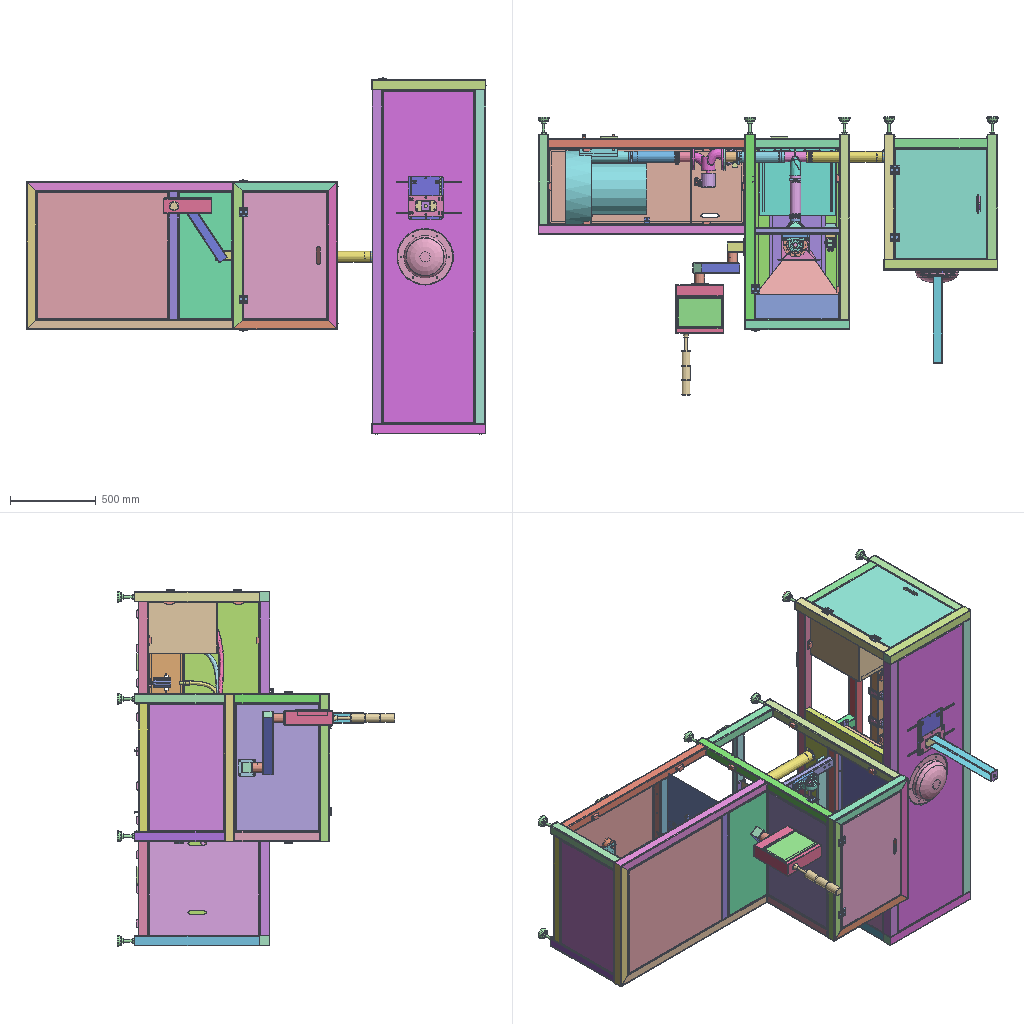Assembly | STEP file | 143 different items | 370 placed | box 2675 x 1617 x 2074 mm
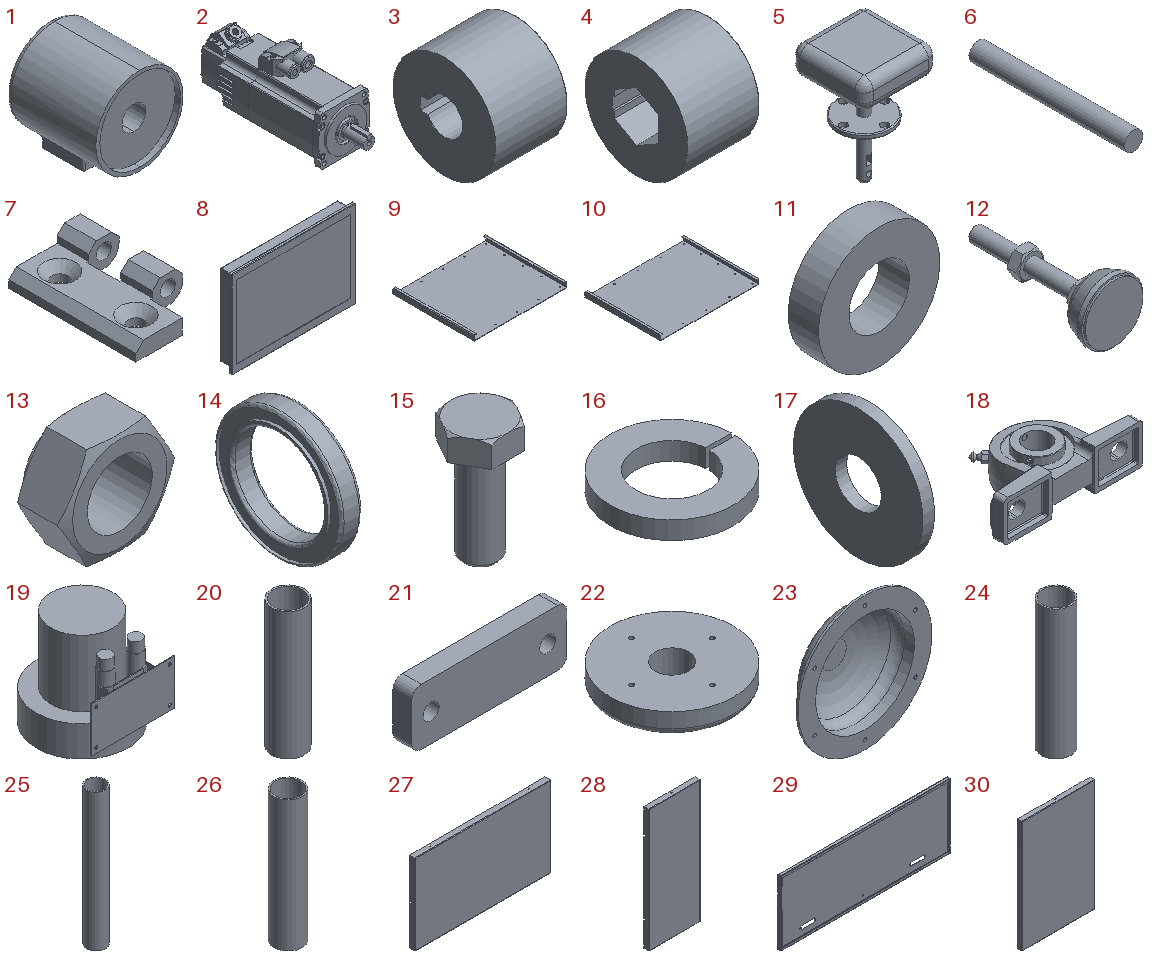Parts list (item | name | quantity | parent item | size | volume):
1 | - | x1 | - | 80 x 82 x 92.2 mm | 393243 mm3
2 | 400W (brake)_1FL60342AF211AB1 | x2 | in JBJ-P-1019-00 | 63.062 x 188.688 x 80 mm | 431591 mm3
3 | ATP40XL050-B-N14 | x1 | in JBJ-P-1019-00 | 28 x 40 x 40 mm | 30210 mm3
4 | ATP40XL050-B-hex socket | x1 | in JBJ-P-1002-00 | 28 x 40 x 40 mm | 27766 mm3
5 | Anemometer | x1 | in Test rig | 80 x 80 x 130 mm | 198324 mm3
6 | C_HHSZ50_pin | x7 | in Hinge 50-hole 30X30_C-HHSZ50 | 6 x 50 x 6 mm | 1414 mm3
7 | C_HHSZ50_pr | x14 | in Hinge 50-hole 30X30_C-HHSZ50 | 31 x 50 x 11.5 mm | 6935 mm3
8 | Display screen | x1 | in Test rig | 274 x 42.7 x 193 mm | 1730721 mm3
9 | Electrical box base plate | x1 | in Test rig | 408 x 355 x 23 mm | 248875 mm3
10 | Electrical box base plate 2 | x1 | in Test rig | 453 x 345 x 23 mm | 265143 mm3
11 | Fixed ring | x1 | in Test rig | 40 x 10 x 40 mm | 9425 mm3
12 | Foot cup | x10 | in JBJ-P-1006-00, Test rig | 65 x 147 x 65 mm | 56921 mm3
13 | GB13681-1992 nut M6 | x8 | in Test rig | 10.835 x 5 x 9.372 mm | 219.571 mm3
14 | GB276-1994 bearing 61806-2Z | x2 | in JBJ-P-1002-00 | 7 x 42 x 42 mm | 3844 mm3
15 | GB5783-2000 bolt M6X16 | x2 | in JBJ-P-1019-00 | 10.89 x 9.431 x 20 mm | 757.875 mm3
16 | GB93-1987 washer 6 | x2 | in JBJ-P-1019-00 | 10.997 x 11 x 1.6 mm | 99.231 mm3
17 | GB96.1-2002 washer 6 | x1 | in JBJ-P-1019-00 | 1.6 x 18 x 18 mm | 355.679 mm3
18 | GBT7810-1995-UCP206 | x3 | in JBJ-P-1002-00 | 165 x 84.83 x 48 mm | 210278 mm3
19 | High-pressure fan RB-81D-2  5.5 | x1 | in Test rig | 445 x 470 x 470 mm | 48196616 mm3
20 | JBJ-P-1000-01 | x1 | in JBJ-P-1000-00 | 64 x 64 x 250 mm | 143728 mm3
21 | JBJ-P-1000-03 | x3 | in JBJ-P-1000-00, Test rig | 165 x 20 x 60 mm | 187204 mm3
22 | JBJ-P-1000-04 | x1 | in Test rig | 198 x 198 x 55 mm | 1265765 mm3
23 | JBJ-P-1000-05 | x1 | in Test rig | 322 x 80 x 322 mm | 568917 mm3
24 | JBJ-P-1000-06 | x1 | in Test rig | 64 x 64 x 280 mm | 160975 mm3
25 | JBJ-P-1000-07 | x1 | in Test rig | 64 x 64 x 470 mm | 270208 mm3
26 | JBJ-P-1000-08 | x1 | in Test rig | 64 x 64 x 298 mm | 171324 mm3
27 | JBJ-P-1000-09 | x1 | in Test rig | 735 x 30 x 435 mm | 461490 mm3
28 | JBJ-P-1000-10 | x1 | in Test rig | 308 x 30 x 735 mm | 340907 mm3
29 | JBJ-P-1000-11 | x1 | in Test rig | 1135 x 20 x 435 mm | 703191 mm3
30 | JBJ-P-1000-12 | x1 | in Test rig | 481 x 30 x 735 mm | 630028 mm3
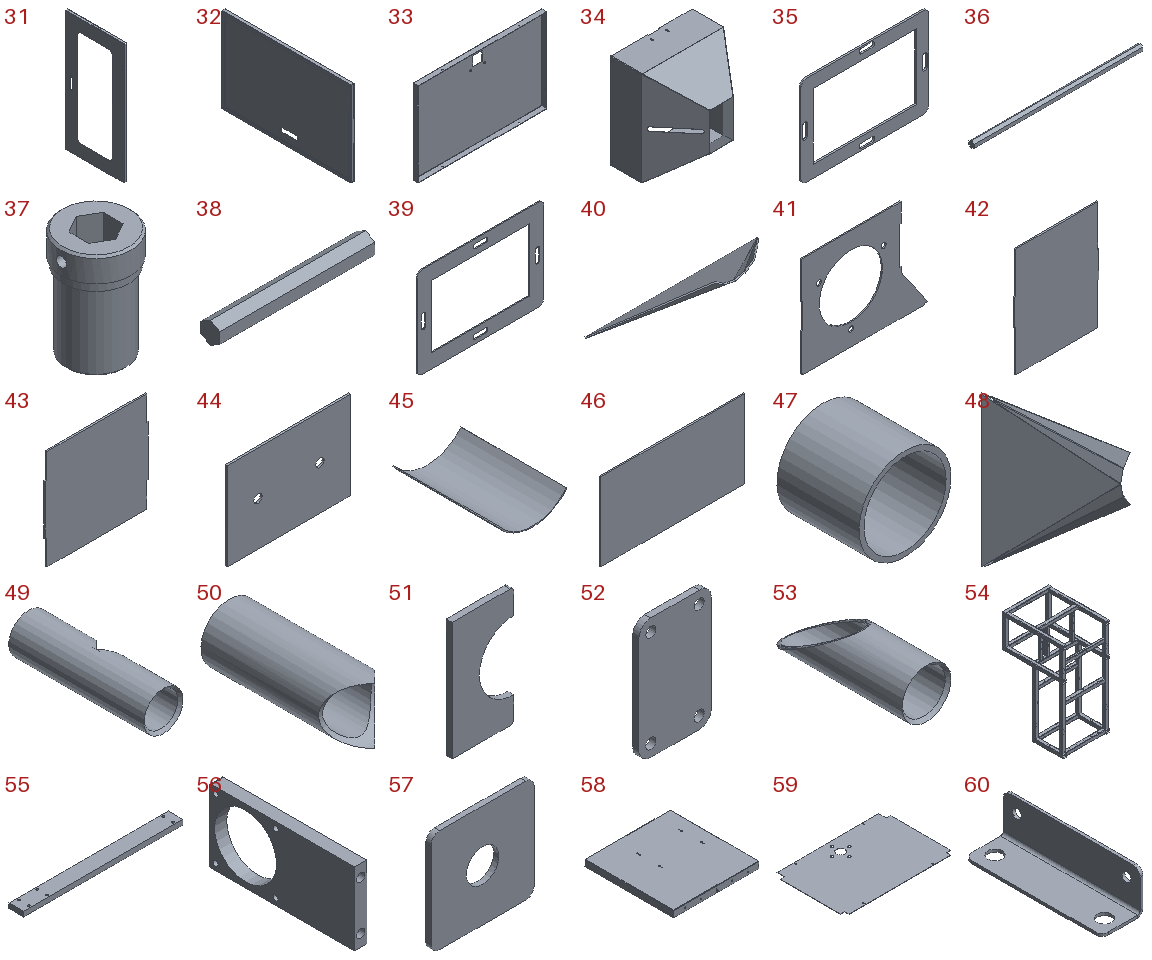31 | JBJ-P-1000-13 | x1 | in Test rig | 20 x 485 x 988 mm | 412527 mm3
32 | JBJ-P-1000-17 | x1 | in Test rig | 20 x 735 x 485 mm | 514895 mm3
33 | JBJ-P-1000-18 | x1 | in Test rig | 735 x 30 x 480 mm | 827406 mm3
34 | JBJ-P-1001-01 | x1 | in JBJ-P-1001-00 | 422 x 360.733 x 487 mm | 588476 mm3
35 | JBJ-P-1001-02 | x1 | in JBJ-P-1001-00 | 241.3 x 3 x 170 mm | 47230 mm3
36 | JBJ-P-1002-05 | x1 | in JBJ-P-1002-00 | 493 x 17 x 19.63 mm | 123389 mm3
37 | JBJ-P-1002-08 | x3 | in JBJ-P-1002-00 | 35 x 35 x 54 mm | 27719 mm3
38 | JBJ-P-1002-09 | x1 | in JBJ-P-1002-00 | 140 x 17 x 19.63 mm | 35039 mm3
39 | JBJ-P-1003-01 | x1 | in JBJ-P-1003-00 | 250 x 2 x 180 mm | 39519 mm3
40 | JBJ-P-1003-010 | x2 | in JBJ-P-1003-00 | 159.641 x 58.923 x 43.35 mm | 8515 mm3
41 | JBJ-P-1003-02 | x2 | in JBJ-P-1003-00 | 203 x 2 x 162 mm | 37833 mm3
42 | JBJ-P-1003-03 | x1 | in JBJ-P-1003-00 | 124 x 2 x 160 mm | 38720 mm3
43 | JBJ-P-1003-04 | x1 | in JBJ-P-1003-00 | 124 x 2 x 120 mm | 29280 mm3
44 | JBJ-P-1003-05 | x1 | in JBJ-P-1003-00 | 120 x 2 x 85 mm | 20199 mm3
45 | JBJ-P-1003-06 | x1 | in JBJ-P-1003-00 | 80.887 x 124 x 20.389 mm | 13687 mm3
46 | JBJ-P-1003-07 | x1 | in JBJ-P-1003-00 | 120 x 1.2 x 65 mm | 9360 mm3
47 | JBJ-P-1003-08 | x1 | in JBJ-P-1003-00 | 56 x 50 x 56 mm | 24976 mm3
48 | JBJ-P-1003-09 | x1 | in JBJ-P-1003-00 | 61.208 x 58.943 x 119.791 mm | 7806 mm3
49 | JBJ-P-1004-01_Default<As Machined> | x1 | in JBJ-P-1004-00 | 58 x 200 x 58 mm | 119017 mm3
50 | JBJ-P-1004-02 | x1 | in JBJ-P-1004-00 | 58 x 150 x 58 mm | 86410 mm3
51 | JBJ-P-1004-03 | x1 | in JBJ-P-1004-00 | 52 x 5 x 100 mm | 19375 mm3
52 | JBJ-P-1004-04 | x1 | in JBJ-P-1004-00 | 60 x 5 x 100 mm | 28436 mm3
53 | JBJ-P-1004-05 | x1 | in JBJ-P-1004-00 | 50 x 146.328 x 50 mm | 46289 mm3
54 | JBJ-P-1006-01_Default<As Machined> | x1 | in JBJ-P-1006-00 | 860 x 1133 x 1810 mm | 13158479 mm3
55 | JBJ-P-1006-02 | x1 | in JBJ-P-1006-00 | 648 x 60 x 20 mm | 770791 mm3
56 | JBJ-P-1006-03 | x1 | in JBJ-P-1006-00 | 10 x 120 x 60 mm | 49516 mm3
57 | JBJ-P-1006-04 | x10 | in JBJ-P-1006-00, Test rig | 60 x 3 x 60 mm | 9885 mm3
58 | JBJ-P-1006-05 | x1 | in Test rig | 735 x 762 x 55 mm | 1423016 mm3
59 | JBJ-P-1006-06 | x1 | in Test rig | 800 x 521 x 2 mm | 813927 mm3
60 | JBJ-P-1006-07 | x2 | in Test rig | 30 x 100 x 30 mm | 10820 mm3
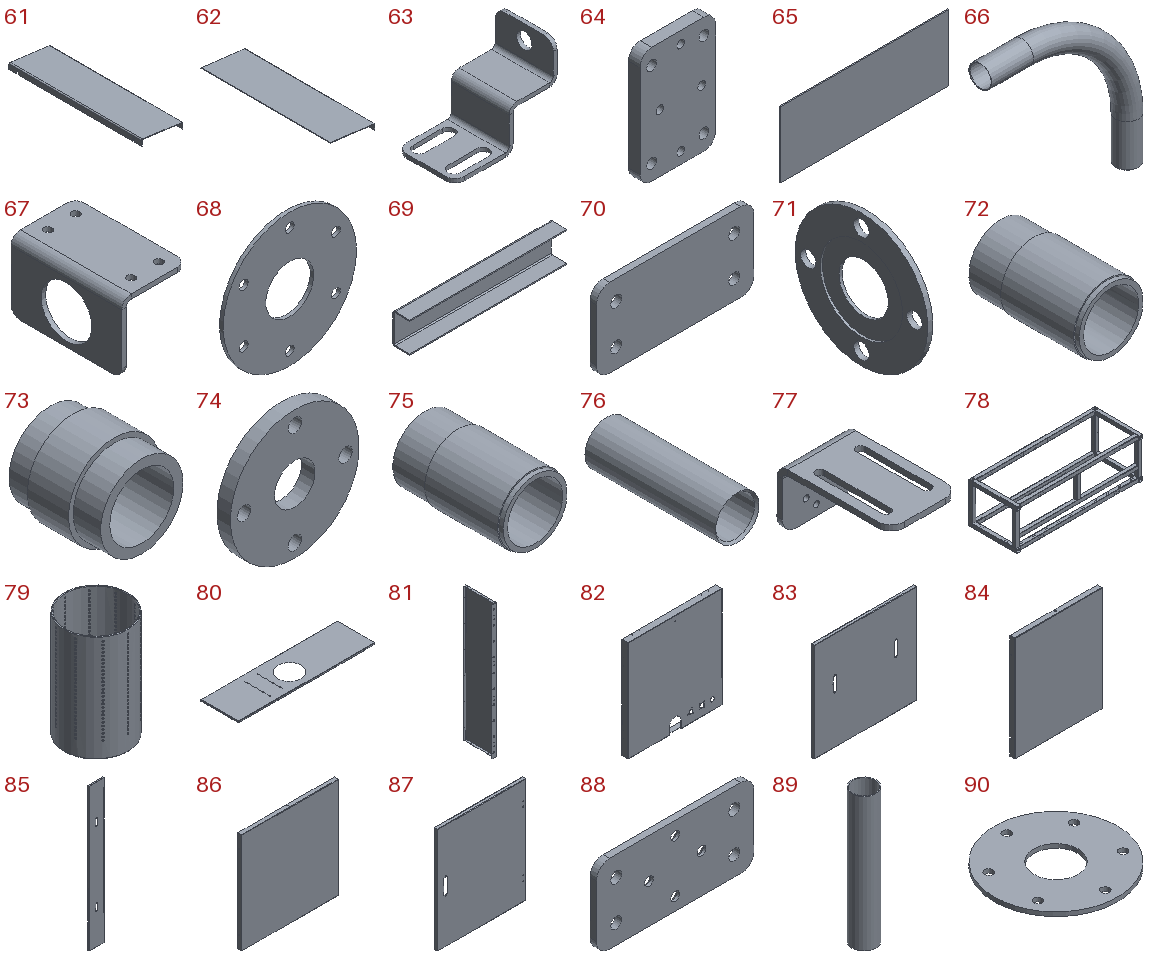61 | JBJ-P-1006-08 | x1 | in Test rig | 152 x 488 x 41.784 mm | 186030 mm3
62 | JBJ-P-1006-09 | x1 | in Test rig | 167 x 488 x 42.231 mm | 182511 mm3
63 | JBJ-P-1006-10 | x3 | in Test rig | 52.8 x 30 x 40 mm | 4550 mm3
64 | JBJ-P-1006-11 | x8 | in Test rig | 65 x 10 x 100 mm | 59980 mm3
65 | JBJ-P-1006-12 | x1 | in Test rig | 828 x 6 x 325 mm | 1614600 mm3
66 | JBJ-P-1007-01 | x1 | in JBJ-P-1007-00 | 377 x 54 x 377 mm | 193491 mm3
67 | JBJ-P-1007-02 | x1 | in JBJ-P-1007-00 | 70 x 120 x 75 mm | 68625 mm3
68 | JBJ-P-1007-03 | x1 | in JBJ-P-1007-00 | 150 x 4 x 150 mm | 59640 mm3
69 | JBJ-P-1007-04 | x1 | in JBJ-P-1007-00 | 300 x 32 x 58 mm | 69255 mm3
70 | JBJ-P-1007-05 | x1 | in JBJ-P-1007-00 | 120 x 5 x 60 mm | 34436 mm3
71 | JBJ-P-1008-01 | x2 | in JBJ-P-1008-00, JBJ-P-1009-00 | 6 x 156 x 156 mm | 80852 mm3
72 | JBJ-P-1008-02 | x1 | in JBJ-P-1008-00 | 60 x 100 x 60 mm | 77175 mm3
73 | JBJ-P-1008-04 | x1 | in JBJ-P-1008-00 | 20 x 20 x 20 mm | 2548 mm3
74 | JBJ-P-1008-05 | x1 | in JBJ-P-1008-00 | 57 x 6 x 57 mm | 13105 mm3
75 | JBJ-P-1009-01 | x1 | in JBJ-P-1009-00 | 60 x 100 x 60 mm | 78768 mm3
76 | JBJ-P-1010-02 | x10 | in Test rig | 20 x 60 x 20 mm | 3552 mm3
77 | JBJ-P-1010-04 | x10 | in Test rig | 50 x 84 x 44 mm | 20932 mm3
78 | JBJ-P-1011-01_Default<As Machined> | x1 | in Test rig | 2060 x 785 x 660 mm | 6965284 mm3
79 | JBJ-P-1011-02 | x10 | in Test rig | 60 x 60 x 100 mm | 25920 mm3
80 | JBJ-P-1011-03 | x1 | in Test rig | 1935 x 535 x 20 mm | 1237179 mm3
81 | JBJ-P-1011-04 | x1 | in Test rig | 61.5 x 440 x 1940 mm | 1252283 mm3
82 | JBJ-P-1011-05a | x1 | in Test rig | 600 x 40 x 643 mm | 566077 mm3
83 | JBJ-P-1011-05b | x1 | in Test rig | 668 x 20 x 643 mm | 606779 mm3
84 | JBJ-P-1011-06 | x1 | in Test rig | 535 x 30 x 640 mm | 489037 mm3
85 | JBJ-P-1011-07 | x1 | in Test rig | 200 x 20 x 1935 mm | 617384 mm3
86 | JBJ-P-1011-08 | x1 | in Test rig | 735 x 30 x 762 mm | 771967 mm3
87 | JBJ-P-1011-09 | x1 | in Test rig | 535 x 20 x 640 mm | 494626 mm3
88 | JBJ-P-1011-10 | x2 | in Test rig | 120 x 5 x 60 mm | 33228 mm3
89 | JBJ-P-1012-01 | x1 | in JBJ-P-1012-00 | 54 x 54 x 300 mm | 98018 mm3
90 | JBJ-P-1012-02 | x1 | in JBJ-P-1012-00 | 150 x 150 x 5 mm | 74550 mm3
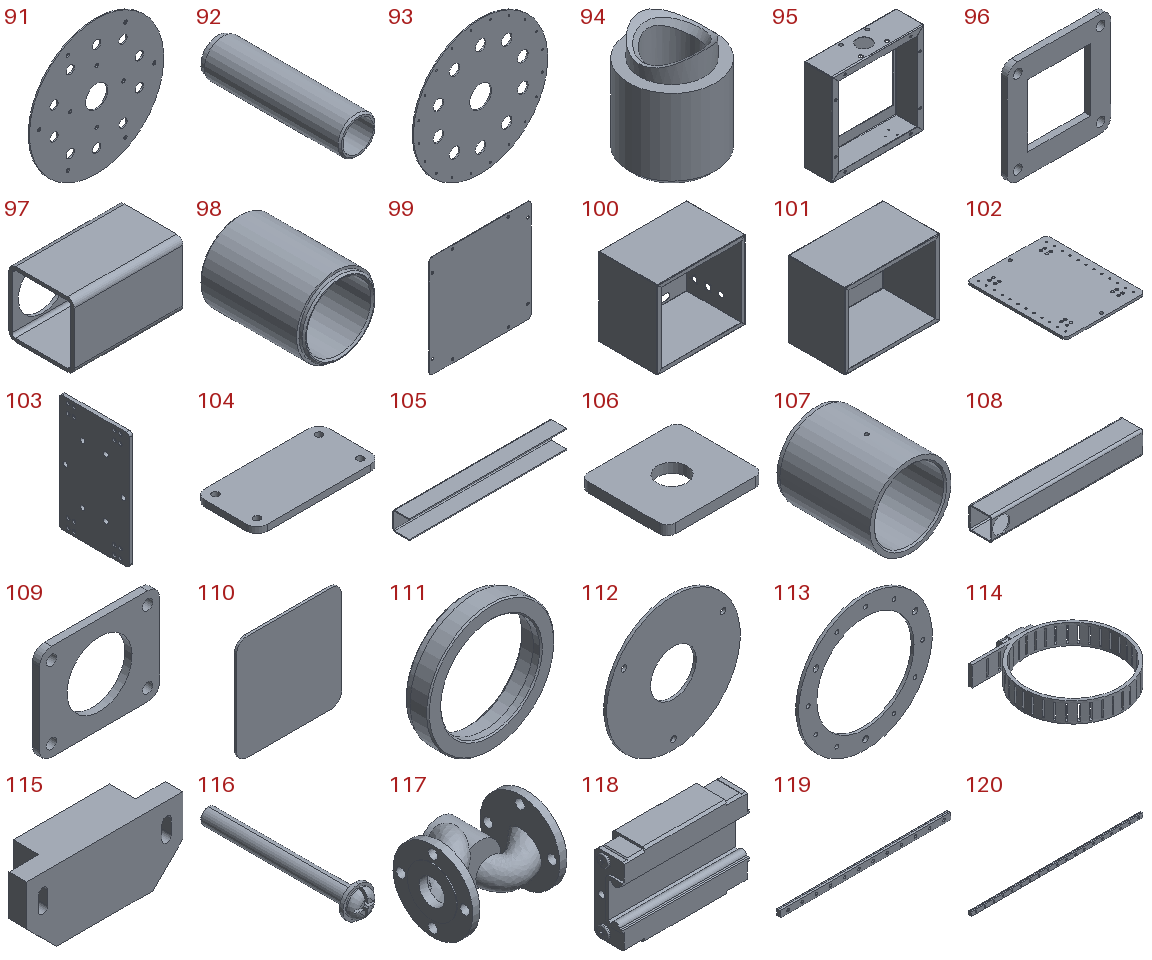91 | JBJ-P-1012-03 | x1 | in JBJ-P-1012-00 | 326 x 3 x 326 mm | 232604 mm3
92 | JBJ-P-1012-04 | x10 | in JBJ-P-1012-00 | 22 x 83 x 22 mm | 9931 mm3
93 | JBJ-P-1012-05 | x1 | in JBJ-P-1012-00 | 330 x 3 x 330 mm | 233037 mm3
94 | JBJ-P-1012-07 | x10 | in JBJ-P-1012-00 | 16 x 16 x 19.292 mm | 2215 mm3
95 | JBJ-P-1013-01 | x1 | in Test rig | 280 x 85 x 280 mm | 166865 mm3
96 | JBJ-P-1013-02 | x1 | in JBJ-P-1013-00 | 100 x 6 x 100 mm | 36162 mm3
97 | JBJ-P-1013-03_Default<As Machined> | x1 | in JBJ-P-1013-00 | 100 x 60 x 60 mm | 61311 mm3
98 | JBJ-P-1013-04 | x2 | in JBJ-P-1013-00, JBJ-P-1016-00 | 48 x 63 x 48 mm | 33905 mm3
99 | JBJ-P-1013-05 | x1 | in Test rig | 274 x 1.2 x 274 mm | 89670 mm3
100 | JBJ-P-1013-06 | x1 | in Test rig | 450 x 300 x 400 mm | 843882 mm3
101 | JBJ-P-1013-07 | x1 | in Test rig | 500 x 300 x 400 mm | 907808 mm3
102 | JBJ-P-1014-01 | x1 | in Test rig | 200 x 250 x 6 mm | 296472 mm3
103 | JBJ-P-1014-02 | x1 | in Test rig | 6 x 120 x 200 mm | 140903 mm3
104 | JBJ-P-1015-01 | x1 | in JBJ-P-1015-00 | 120 x 60 x 6 mm | 41889 mm3
105 | JBJ-P-1015-02_Default<As Machined> | x1 | in JBJ-P-1015-00 | 500 x 54 x 60 mm | 237206 mm3
106 | JBJ-P-1015-03 | x1 | in JBJ-P-1015-00 | 60 x 54 x 6 mm | 17698 mm3
107 | JBJ-P-1016-01 | x2 | in JBJ-P-1016-00, JBJ-P-1017-00 | 56 x 65 x 56 mm | 41860 mm3
108 | JBJ-P-1016-02_Default<As Machined> | x1 | in JBJ-P-1016-00 | 400 x 60 x 60 mm | 252664 mm3
109 | JBJ-P-1017-01 | x1 | in JBJ-P-1017-00 | 100 x 6 x 80 mm | 32382 mm3
110 | JBJ-P-1017-02 | x7 | in JBJ-P-1013-00, JBJ-P-1016-00, Test rig | 60 x 1.2 x 60 mm | 4283 mm3
111 | JBJ-P-1018-01 | x2 | in JBJ-P-1018-00 | 50 x 10 x 50 mm | 5771 mm3
112 | JBJ-P-1018-02 | x2 | in JBJ-P-1018-00 | 140 x 3 x 140 mm | 40498 mm3
113 | JBJ-P-1018-03 | x2 | in JBJ-P-1018-00 | 140 x 3 x 140 mm | 21074 mm3
114 | JBT 8870—1999 70-90 | x8 | in JBJ-P-1000-00, Test rig | 67 x 72 x 13 mm | 5818 mm3
115 | Large white magnetic mount | x41 | in Test rig | 57.5 x 16 x 26 mm | 17347 mm3
116 | - | x1 | - | 6 x 30.7 x 6 mm | 238.696 mm3
117 | Part 11 | x1 | in ZCZP-1P-K-Z DN50 | 188 x 178 x 156 mm | 934142 mm3
118 | RSR9KM1-2 | x8 | in Slide rail RSR9KM1-250, Slide rail RSR9KM1-500 | 30.8 x 7.8 x 20 mm | 3450 mm3
119 | RSR9KM1-250-1 | x2 | in Slide rail RSR9KM1-250 | 240 x 5.5 x 9 mm | 9857 mm3
120 | RSR9KM1-500-1 | x2 | in Slide rail RSR9KM1-500 | 380 x 5.5 x 9 mm | 15608 mm3
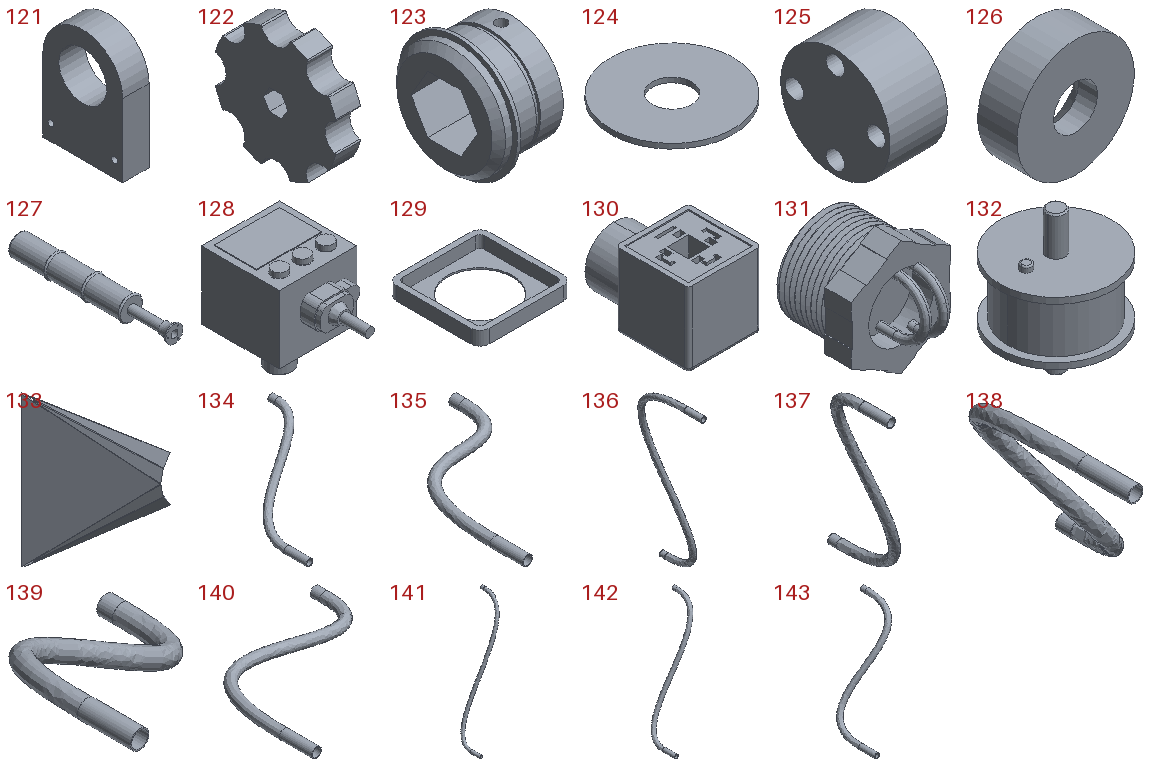121 | Ring photoelectric switch | x10 | in Test rig | 20 x 60 x 91 mm | 73356 mm3
122 | Segmented slotted wheel | x6 | in Slotted wheel assembly | 20 x 96.923 x 96.923 mm | 125193 mm3
123 | Slotted wheel end cap | x2 | in Slotted wheel assembly | 20 x 35 x 35 mm | 9444 mm3
124 | Slotted wheel end cap 2 | x2 | in JBJ-P-1002-00 | 100 x 100 x 4 mm | 28199 mm3
125 | Small compression-type pressure sensor LFC-20P | x10 | in Test rig | 11 x 20 x 20 mm | 3302 mm3
126 | Strong magnet | x10 | in Test rig | 12 x 4 x 12 mm | 350.045 mm3
127 | Three-colour light | x1 | in Test rig | 56 x 361 x 56 mm | 538523 mm3
128 | _ZSE40AF-01-A_BODY(0).stp | x11 | in ZSE40AF-01-R-MA-X501(0).stp | 30 x 50 x 42.2 mm | 26079 mm3
129 | - | x1 | - | 30.5 x 30.5 x 4.5 mm | 1063 mm3
130 | - | x1 | - | 26.7 x 40.7 x 27.46 mm | 19718 mm3
131 | - | x1 | - | 18.7 x 20.75 x 21.593 mm | 2111 mm3
132 | lt-x-8000-04 | x4 | in Test rig | - | -
133 | Mirror JBJ-P-1003-09 | x1 | in JBJ-P-1003-00 | 61.208 x 58.943 x 119.791 mm | 7806 mm3
134 | Part 10^JBJ-F-0000-00 | x1 | in Test rig | 298.36 x 417.992 x 226.424 mm | 91020 mm3
135 | Part 11^JBJ-F-0000-00 | x1 | in Test rig | 248.297 x 414.992 x 71.5 mm | 86273 mm3
136 | Part 2^JBJ-F-0000-00 | x1 | in Test rig | 234.291 x 415.992 x 914.606 mm | 198661 mm3
137 | Part 3^JBJ-F-0000-00 | x1 | in Test rig | 261.691 x 414.992 x 653.065 mm | 148714 mm3
138 | Part 4^JBJ-F-0000-00 | x1 | in Test rig | 320.031 x 414.992 x 419.382 mm | 125699 mm3
139 | Part 5^JBJ-F-0000-00 | x1 | in Test rig | 391.028 x 414.992 x 230.424 mm | 128093 mm3
140 | Part 6^JBJ-F-0000-00 | x1 | in Test rig | 437.091 x 414.992 x 71.5 mm | 113332 mm3
141 | Part 7^JBJ-F-0000-00 | x1 | in Test rig | 451.097 x 417.992 x 914.606 mm | 190642 mm3
142 | Part 8^JBJ-F-0000-00 | x1 | in Test rig | 423.697 x 414.992 x 653.065 mm | 153249 mm3
143 | Part 9^JBJ-F-0000-00 | x1 | in Test rig | 365.356 x 414.992 x 419.382 mm | 128951 mm3